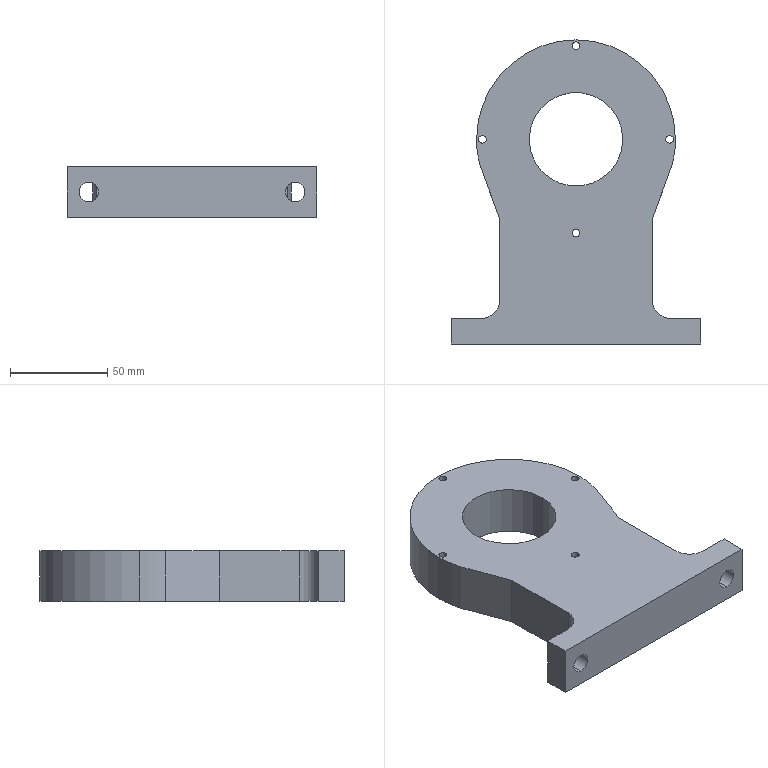Part | NX | features BREP 1 | 1 solid | 32 faces | box 128 x 156 x 26 mm | volume 302066 mm3 | cylinder 19 | plane 13 | commonest cylinder face diameters 4 x8 10 x4 102 x3 20 x2 48 x2
STEP:
#1=CARTESIAN_POINT('',(-50.,32.864,0.));
#2=VERTEX_POINT('',#1);
#3=CARTESIAN_POINT('',(-46.,32.864,0.));
#4=VERTEX_POINT('',#3);
#5=CARTESIAN_POINT('',(-48.,32.864,0.));
#6=DIRECTION('',(0.,0.,1.));
#7=DIRECTION('',(-1.,0.,0.));
#8=AXIS2_PLACEMENT_3D('',#5,#6,#7);
#9=CIRCLE('',#8,2.);
#10=EDGE_CURVE('',#2,#4,#9,.T.);
#11=ORIENTED_EDGE('',*,*,#10,.F.);
#12=CARTESIAN_POINT('',(-50.,32.864,26.));
#13=VERTEX_POINT('',#12);
#14=CARTESIAN_POINT('',(-50.,32.864,-0.001));
#15=DIRECTION('',(0.,0.,1.));
#16=VECTOR('',#15,1000.);
#17=LINE('',#14,#16);
#18=EDGE_CURVE('',#2,#13,#17,.T.);
#19=ORIENTED_EDGE('',*,*,#18,.T.);
#20=CARTESIAN_POINT('',(-46.,32.864,26.));
#21=VERTEX_POINT('',#20);
#22=CARTESIAN_POINT('',(-48.,32.864,26.));
#23=DIRECTION('',(0.,0.,1.));
#24=DIRECTION('',(1.,0.,0.));
#25=AXIS2_PLACEMENT_3D('',#22,#23,#24);
#26=CIRCLE('',#25,2.);
#27=EDGE_CURVE('',#13,#21,#26,.T.);
#28=ORIENTED_EDGE('',*,*,#27,.T.);
#29=CARTESIAN_POINT('',(-46.,32.864,-0.001));
#30=DIRECTION('',(0.,0.,1.));
#31=VECTOR('',#30,1000.);
#32=LINE('',#29,#31);
#33=EDGE_CURVE('',#4,#21,#32,.T.);
#34=ORIENTED_EDGE('',*,*,#33,.F.);
#35=EDGE_LOOP('',(#11,#19,#28,#34));
#36=FACE_BOUND('',#35,.T.);
#37=CARTESIAN_POINT('',(-48.,32.864,-0.001));
#38=DIRECTION('',(0.,0.,1.));
#39=DIRECTION('',(-1.,0.,0.));
#40=AXIS2_PLACEMENT_3D('',#37,#38,#39);
#41=CYLINDRICAL_SURFACE('',#40,2.);
#42=ADVANCED_FACE('',(#36),#41,.F.);
#43=CARTESIAN_POINT('',(-2.,-15.136,0.));
#44=VERTEX_POINT('',#43);
#45=CARTESIAN_POINT('',(2.,-15.136,0.));
#46=VERTEX_POINT('',#45);
#47=CARTESIAN_POINT('',(0.,-15.136,0.));
#48=DIRECTION('',(0.,0.,1.));
#49=DIRECTION('',(-1.,0.,0.));
#50=AXIS2_PLACEMENT_3D('',#47,#48,#49);
#51=CIRCLE('',#50,2.);
#52=EDGE_CURVE('',#44,#46,#51,.T.);
#53=ORIENTED_EDGE('',*,*,#52,.F.);
#54=CARTESIAN_POINT('',(-2.,-15.136,26.));
#55=VERTEX_POINT('',#54);
#56=CARTESIAN_POINT('',(-2.,-15.136,-0.001));
#57=DIRECTION('',(0.,0.,1.));
#58=VECTOR('',#57,1000.);
#59=LINE('',#56,#58);
#60=EDGE_CURVE('',#44,#55,#59,.T.);
#61=ORIENTED_EDGE('',*,*,#60,.T.);
#62=CARTESIAN_POINT('',(2.,-15.136,26.));
#63=VERTEX_POINT('',#62);
#64=CARTESIAN_POINT('',(0.,-15.136,26.));
#65=DIRECTION('',(0.,0.,1.));
#66=DIRECTION('',(1.,0.,0.));
#67=AXIS2_PLACEMENT_3D('',#64,#65,#66);
#68=CIRCLE('',#67,2.);
#69=EDGE_CURVE('',#55,#63,#68,.T.);
#70=ORIENTED_EDGE('',*,*,#69,.T.);
#71=CARTESIAN_POINT('',(2.,-15.136,-0.001));
#72=DIRECTION('',(0.,0.,1.));
#73=VECTOR('',#72,1000.);
#74=LINE('',#71,#73);
#75=EDGE_CURVE('',#46,#63,#74,.T.);
#76=ORIENTED_EDGE('',*,*,#75,.F.);
#77=EDGE_LOOP('',(#53,#61,#70,#76));
#78=FACE_BOUND('',#77,.T.);
#79=CARTESIAN_POINT('',(0.,-15.136,-0.001));
#80=DIRECTION('',(0.,0.,1.));
#81=DIRECTION('',(-1.,0.,0.));
#82=AXIS2_PLACEMENT_3D('',#79,#80,#81);
#83=CYLINDRICAL_SURFACE('',#82,2.);
#84=ADVANCED_FACE('',(#78),#83,.F.);
#85=CARTESIAN_POINT('',(46.,32.864,0.));
#86=VERTEX_POINT('',#85);
#87=CARTESIAN_POINT('',(50.,32.864,0.));
#88=VERTEX_POINT('',#87);
#89=CARTESIAN_POINT('',(48.,32.864,0.));
#90=DIRECTION('',(0.,0.,1.));
#91=DIRECTION('',(-1.,0.,0.));
#92=AXIS2_PLACEMENT_3D('',#89,#90,#91);
#93=CIRCLE('',#92,2.);
#94=EDGE_CURVE('',#86,#88,#93,.T.);
#95=ORIENTED_EDGE('',*,*,#94,.F.);
#96=CARTESIAN_POINT('',(46.,32.864,26.));
#97=VERTEX_POINT('',#96);
#98=CARTESIAN_POINT('',(46.,32.864,-0.001));
#99=DIRECTION('',(0.,0.,1.));
#100=VECTOR('',#99,1000.);
#101=LINE('',#98,#100);
#102=EDGE_CURVE('',#86,#97,#101,.T.);
#103=ORIENTED_EDGE('',*,*,#102,.T.);
#104=CARTESIAN_POINT('',(50.,32.864,26.));
#105=VERTEX_POINT('',#104);
#106=CARTESIAN_POINT('',(48.,32.864,26.));
#107=DIRECTION('',(0.,0.,1.));
#108=DIRECTION('',(1.,0.,0.));
#109=AXIS2_PLACEMENT_3D('',#106,#107,#108);
#110=CIRCLE('',#109,2.);
#111=EDGE_CURVE('',#97,#105,#110,.T.);
#112=ORIENTED_EDGE('',*,*,#111,.T.);
#113=CARTESIAN_POINT('',(50.,32.864,-0.001));
#114=DIRECTION('',(0.,0.,1.));
#115=VECTOR('',#114,1000.);
#116=LINE('',#113,#115);
#117=EDGE_CURVE('',#88,#105,#116,.T.);
#118=ORIENTED_EDGE('',*,*,#117,.F.);
#119=EDGE_LOOP('',(#95,#103,#112,#118));
#120=FACE_BOUND('',#119,.T.);
#121=CARTESIAN_POINT('',(48.,32.864,-0.001));
#122=DIRECTION('',(0.,0.,1.));
#123=DIRECTION('',(-1.,0.,0.));
#124=AXIS2_PLACEMENT_3D('',#121,#122,#123);
#125=CYLINDRICAL_SURFACE('',#124,2.);
#126=ADVANCED_FACE('',(#120),#125,.F.);
#127=CARTESIAN_POINT('',(-2.,80.864,0.));
#128=VERTEX_POINT('',#127);
#129=CARTESIAN_POINT('',(2.,80.864,0.));
#130=VERTEX_POINT('',#129);
#131=CARTESIAN_POINT('',(0.,80.864,0.));
#132=DIRECTION('',(0.,0.,1.));
#133=DIRECTION('',(-1.,0.,0.));
#134=AXIS2_PLACEMENT_3D('',#131,#132,#133);
#135=CIRCLE('',#134,2.);
#136=EDGE_CURVE('',#128,#130,#135,.T.);
#137=ORIENTED_EDGE('',*,*,#136,.F.);
#138=CARTESIAN_POINT('',(-2.,80.864,26.));
#139=VERTEX_POINT('',#138);
#140=CARTESIAN_POINT('',(-2.,80.864,-0.001));
#141=DIRECTION('',(0.,0.,1.));
#142=VECTOR('',#141,1000.);
#143=LINE('',#140,#142);
#144=EDGE_CURVE('',#128,#139,#143,.T.);
#145=ORIENTED_EDGE('',*,*,#144,.T.);
#146=CARTESIAN_POINT('',(2.,80.864,26.));
#147=VERTEX_POINT('',#146);
#148=CARTESIAN_POINT('',(0.,80.864,26.));
#149=DIRECTION('',(0.,0.,1.));
#150=DIRECTION('',(1.,0.,0.));
#151=AXIS2_PLACEMENT_3D('',#148,#149,#150);
#152=CIRCLE('',#151,2.);
#153=EDGE_CURVE('',#139,#147,#152,.T.);
#154=ORIENTED_EDGE('',*,*,#153,.T.);
#155=CARTESIAN_POINT('',(2.,80.864,-0.001));
#156=DIRECTION('',(0.,0.,1.));
#157=VECTOR('',#156,1000.);
#158=LINE('',#155,#157);
#159=EDGE_CURVE('',#130,#147,#158,.T.);
#160=ORIENTED_EDGE('',*,*,#159,.F.);
#161=EDGE_LOOP('',(#137,#145,#154,#160));
#162=FACE_BOUND('',#161,.T.);
#163=CARTESIAN_POINT('',(0.,80.864,-0.001));
#164=DIRECTION('',(0.,0.,1.));
#165=DIRECTION('',(-1.,0.,0.));
#166=AXIS2_PLACEMENT_3D('',#163,#164,#165);
#167=CYLINDRICAL_SURFACE('',#166,2.);
#168=ADVANCED_FACE('',(#162),#167,.F.);
#169=CARTESIAN_POINT('',(53.,-72.136,18.));
#170=VERTEX_POINT('',#169);
#171=CARTESIAN_POINT('',(53.,-72.136,8.));
#172=VERTEX_POINT('',#171);
#173=CARTESIAN_POINT('',(53.,-72.136,13.));
#174=DIRECTION('',(0.,-1.,0.));
#175=DIRECTION('',(0.,0.,1.));
#176=AXIS2_PLACEMENT_3D('',#173,#174,#175);
#177=CIRCLE('',#176,5.);
#178=EDGE_CURVE('',#170,#172,#177,.T.);
#179=ORIENTED_EDGE('',*,*,#178,.T.);
#180=CARTESIAN_POINT('',(53.,-59.136,8.));
#181=VERTEX_POINT('',#180);
#182=CARTESIAN_POINT('',(53.,-72.137,8.));
#183=DIRECTION('',(0.,1.,0.));
#184=VECTOR('',#183,1000.);
#185=LINE('',#182,#184);
#186=EDGE_CURVE('',#172,#181,#185,.T.);
#187=ORIENTED_EDGE('',*,*,#186,.T.);
#188=CARTESIAN_POINT('',(49.,-59.136,10.));
#189=VERTEX_POINT('',#188);
#190=CARTESIAN_POINT('',(53.,-59.136,13.));
#191=DIRECTION('',(0.,1.,0.));
#192=DIRECTION('',(0.,0.,1.));
#193=AXIS2_PLACEMENT_3D('',#190,#191,#192);
#194=CIRCLE('',#193,5.);
#195=EDGE_CURVE('',#181,#189,#194,.T.);
#196=ORIENTED_EDGE('',*,*,#195,.T.);
#197=CARTESIAN_POINT('',(49.,-59.136,16.));
#198=VERTEX_POINT('',#197);
#199=CARTESIAN_POINT('',(53.,-59.136,13.));
#200=DIRECTION('',(0.,1.,0.));
#201=DIRECTION('',(0.,0.,1.));
#202=AXIS2_PLACEMENT_3D('',#199,#200,#201);
#203=CIRCLE('',#202,5.);
#204=EDGE_CURVE('',#189,#198,#203,.T.);
#205=ORIENTED_EDGE('',*,*,#204,.T.);
#206=CARTESIAN_POINT('',(53.,-59.136,18.));
#207=VERTEX_POINT('',#206);
#208=CARTESIAN_POINT('',(53.,-59.136,13.));
#209=DIRECTION('',(0.,1.,0.));
#210=DIRECTION('',(0.,0.,1.));
#211=AXIS2_PLACEMENT_3D('',#208,#209,#210);
#212=CIRCLE('',#211,5.);
#213=EDGE_CURVE('',#198,#207,#212,.T.);
#214=ORIENTED_EDGE('',*,*,#213,.T.);
#215=CARTESIAN_POINT('',(53.,-72.137,18.));
#216=DIRECTION('',(0.,1.,0.));
#217=VECTOR('',#216,1000.);
#218=LINE('',#215,#217);
#219=EDGE_CURVE('',#170,#207,#218,.T.);
#220=ORIENTED_EDGE('',*,*,#219,.F.);
#221=EDGE_LOOP('',(#179,#187,#196,#205,#214,#220));
#222=FACE_BOUND('',#221,.T.);
#223=CARTESIAN_POINT('',(53.,-72.137,13.));
#224=DIRECTION('',(0.,1.,0.));
#225=DIRECTION('',(0.,0.,-1.));
#226=AXIS2_PLACEMENT_3D('',#223,#224,#225);
#227=CYLINDRICAL_SURFACE('',#226,5.);
#228=ADVANCED_FACE('',(#222),#227,.F.);
#229=CARTESIAN_POINT('',(-53.,-72.136,18.));
#230=VERTEX_POINT('',#229);
#231=CARTESIAN_POINT('',(-53.,-72.136,8.));
#232=VERTEX_POINT('',#231);
#233=CARTESIAN_POINT('',(-53.,-72.136,13.));
#234=DIRECTION('',(0.,-1.,0.));
#235=DIRECTION('',(0.,0.,1.));
#236=AXIS2_PLACEMENT_3D('',#233,#234,#235);
#237=CIRCLE('',#236,5.);
#238=EDGE_CURVE('',#230,#232,#237,.T.);
#239=ORIENTED_EDGE('',*,*,#238,.T.);
#240=CARTESIAN_POINT('',(-53.,-59.136,8.));
#241=VERTEX_POINT('',#240);
#242=CARTESIAN_POINT('',(-53.,-72.137,8.));
#243=DIRECTION('',(0.,1.,0.));
#244=VECTOR('',#243,1000.);
#245=LINE('',#242,#244);
#246=EDGE_CURVE('',#232,#241,#245,.T.);
#247=ORIENTED_EDGE('',*,*,#246,.T.);
#248=CARTESIAN_POINT('',(-53.,-59.136,18.));
#249=VERTEX_POINT('',#248);
#250=CARTESIAN_POINT('',(-53.,-59.136,13.));
#251=DIRECTION('',(0.,1.,0.));
#252=DIRECTION('',(0.,0.,1.));
#253=AXIS2_PLACEMENT_3D('',#250,#251,#252);
#254=CIRCLE('',#253,5.);
#255=EDGE_CURVE('',#241,#249,#254,.T.);
#256=ORIENTED_EDGE('',*,*,#255,.T.);
#257=CARTESIAN_POINT('',(-53.,-72.137,18.));
#258=DIRECTION('',(0.,1.,0.));
#259=VECTOR('',#258,1000.);
#260=LINE('',#257,#259);
#261=EDGE_CURVE('',#230,#249,#260,.T.);
#262=ORIENTED_EDGE('',*,*,#261,.F.);
#263=EDGE_LOOP('',(#239,#247,#256,#262));
#264=FACE_BOUND('',#263,.T.);
#265=CARTESIAN_POINT('',(-53.,-72.137,13.));
#266=DIRECTION('',(0.,1.,0.));
#267=DIRECTION('',(0.,0.,-1.));
#268=AXIS2_PLACEMENT_3D('',#265,#266,#267);
#269=CYLINDRICAL_SURFACE('',#268,5.);
#270=ADVANCED_FACE('',(#264),#269,.F.);
#271=CARTESIAN_POINT('',(-24.,32.864,26.));
#272=VERTEX_POINT('',#271);
#273=CARTESIAN_POINT('',(24.,32.864,26.));
#274=VERTEX_POINT('',#273);
#275=CARTESIAN_POINT('',(0.,32.864,26.));
#276=DIRECTION('',(0.,0.,1.));
#277=DIRECTION('',(1.,0.,0.));
#278=AXIS2_PLACEMENT_3D('',#275,#276,#277);
#279=CIRCLE('',#278,24.);
#280=EDGE_CURVE('',#272,#274,#279,.T.);
#281=ORIENTED_EDGE('',*,*,#280,.T.);
#282=CARTESIAN_POINT('',(24.,32.864,0.));
#283=VERTEX_POINT('',#282);
#284=CARTESIAN_POINT('',(24.,32.864,26.));
#285=DIRECTION('',(0.,0.,-1.));
#286=VECTOR('',#285,1000.);
#287=LINE('',#284,#286);
#288=EDGE_CURVE('',#283,#274,#287,.F.);
#289=ORIENTED_EDGE('',*,*,#288,.F.);
#290=CARTESIAN_POINT('',(-24.,32.864,0.));
#291=VERTEX_POINT('',#290);
#292=CARTESIAN_POINT('',(0.,32.864,0.));
#293=DIRECTION('',(0.,0.,1.));
#294=DIRECTION('',(1.,0.,0.));
#295=AXIS2_PLACEMENT_3D('',#292,#293,#294);
#296=CIRCLE('',#295,24.);
#297=EDGE_CURVE('',#291,#283,#296,.T.);
#298=ORIENTED_EDGE('',*,*,#297,.F.);
#299=CARTESIAN_POINT('',(-24.,32.864,26.));
#300=DIRECTION('',(0.,0.,-1.));
#301=VECTOR('',#300,1000.);
#302=LINE('',#299,#301);
#303=EDGE_CURVE('',#291,#272,#302,.F.);
#304=ORIENTED_EDGE('',*,*,#303,.T.);
#305=EDGE_LOOP('',(#281,#289,#298,#304));
#306=FACE_BOUND('',#305,.T.);
#307=CARTESIAN_POINT('',(0.,32.864,26.));
#308=DIRECTION('',(0.,0.,-1.));
#309=DIRECTION('',(1.,0.,0.));
#310=AXIS2_PLACEMENT_3D('',#307,#308,#309);
#311=CYLINDRICAL_SURFACE('',#310,24.);
#312=ADVANCED_FACE('',(#306),#311,.F.);
#313=CARTESIAN_POINT('',(51.,32.864,26.));
#314=VERTEX_POINT('',#313);
#315=CARTESIAN_POINT('',(-51.,32.864,26.));
#316=VERTEX_POINT('',#315);
#317=CARTESIAN_POINT('',(0.,32.864,26.));
#318=DIRECTION('',(0.,0.,1.));
#319=DIRECTION('',(1.,0.,0.));
#320=AXIS2_PLACEMENT_3D('',#317,#318,#319);
#321=CIRCLE('',#320,51.);
#322=EDGE_CURVE('',#314,#316,#321,.T.);
#323=ORIENTED_EDGE('',*,*,#322,.F.);
#324=CARTESIAN_POINT('',(51.,32.864,0.));
#325=VERTEX_POINT('',#324);
#326=CARTESIAN_POINT('',(51.,32.864,26.));
#327=DIRECTION('',(0.,0.,-1.));
#328=VECTOR('',#327,1000.);
#329=LINE('',#326,#328);
#330=EDGE_CURVE('',#314,#325,#329,.T.);
#331=ORIENTED_EDGE('',*,*,#330,.T.);
#332=CARTESIAN_POINT('',(-51.,32.864,0.));
#333=VERTEX_POINT('',#332);
#334=CARTESIAN_POINT('',(0.,32.864,0.));
#335=DIRECTION('',(0.,0.,1.));
#336=DIRECTION('',(1.,0.,0.));
#337=AXIS2_PLACEMENT_3D('',#334,#335,#336);
#338=CIRCLE('',#337,51.);
#339=EDGE_CURVE('',#325,#333,#338,.T.);
#340=ORIENTED_EDGE('',*,*,#339,.T.);
#341=CARTESIAN_POINT('',(-51.,32.864,26.));
#342=DIRECTION('',(0.,0.,-1.));
#343=VECTOR('',#342,1000.);
#344=LINE('',#341,#343);
#345=EDGE_CURVE('',#316,#333,#344,.T.);
#346=ORIENTED_EDGE('',*,*,#345,.F.);
#347=EDGE_LOOP('',(#323,#331,#340,#346));
#348=FACE_BOUND('',#347,.T.);
#349=CARTESIAN_POINT('',(0.,32.864,26.));
#350=DIRECTION('',(0.,0.,-1.));
#351=DIRECTION('',(1.,0.,0.));
#352=AXIS2_PLACEMENT_3D('',#349,#350,#351);
#353=CYLINDRICAL_SURFACE('',#352,51.);
#354=ADVANCED_FACE('',(#348),#353,.T.);
#355=CARTESIAN_POINT('',(-49.179,19.357,26.));
#356=VERTEX_POINT('',#355);
#357=CARTESIAN_POINT('',(0.,32.864,26.));
#358=DIRECTION('',(0.,0.,1.));
#359=DIRECTION('',(1.,0.,0.));
#360=AXIS2_PLACEMENT_3D('',#357,#358,#359);
#361=CIRCLE('',#360,51.);
#362=EDGE_CURVE('',#316,#356,#361,.T.);
#363=ORIENTED_EDGE('',*,*,#362,.F.);
#364=ORIENTED_EDGE('',*,*,#345,.T.);
#365=CARTESIAN_POINT('',(-49.179,19.357,0.));
#366=VERTEX_POINT('',#365);
#367=CARTESIAN_POINT('',(0.,32.864,0.));
#368=DIRECTION('',(0.,0.,1.));
#369=DIRECTION('',(1.,0.,0.));
#370=AXIS2_PLACEMENT_3D('',#367,#368,#369);
#371=CIRCLE('',#370,51.);
#372=EDGE_CURVE('',#333,#366,#371,.T.);
#373=ORIENTED_EDGE('',*,*,#372,.T.);
#374=CARTESIAN_POINT('',(-49.179,19.357,26.));
#375=DIRECTION('',(0.,0.,-1.));
#376=VECTOR('',#375,1000.);
#377=LINE('',#374,#376);
#378=EDGE_CURVE('',#356,#366,#377,.T.);
#379=ORIENTED_EDGE('',*,*,#378,.F.);
#380=EDGE_LOOP('',(#363,#364,#373,#379));
#381=FACE_BOUND('',#380,.T.);
#382=CARTESIAN_POINT('',(0.,32.864,26.));
#383=DIRECTION('',(0.,0.,-1.));
#384=DIRECTION('',(1.,0.,0.));
#385=AXIS2_PLACEMENT_3D('',#382,#383,#384);
#386=CYLINDRICAL_SURFACE('',#385,51.);
#387=ADVANCED_FACE('',(#381),#386,.T.);
#388=CARTESIAN_POINT('',(39.,-49.136,26.));
#389=VERTEX_POINT('',#388);
#390=CARTESIAN_POINT('',(39.,-8.136,26.));
#391=VERTEX_POINT('',#390);
#392=CARTESIAN_POINT('',(39.,-8.136,26.));
#393=DIRECTION('',(0.,1.,0.));
#394=VECTOR('',#393,1000.);
#395=LINE('',#392,#394);
#396=EDGE_CURVE('',#389,#391,#395,.T.);
#397=ORIENTED_EDGE('',*,*,#396,.T.);
#398=CARTESIAN_POINT('',(49.179,19.357,26.));
#399=VERTEX_POINT('',#398);
#400=CARTESIAN_POINT('',(39.,-8.136,26.));
#401=DIRECTION('',(0.3472,0.9378,0.));
#402=VECTOR('',#401,1000.);
#403=LINE('',#400,#402);
#404=EDGE_CURVE('',#391,#399,#403,.T.);
#405=ORIENTED_EDGE('',*,*,#404,.T.);
#406=CARTESIAN_POINT('',(0.,32.864,26.));
#407=DIRECTION('',(0.,0.,1.));
#408=DIRECTION('',(1.,0.,0.));
#409=AXIS2_PLACEMENT_3D('',#406,#407,#408);
#410=CIRCLE('',#409,51.);
#411=EDGE_CURVE('',#399,#314,#410,.T.);
#412=ORIENTED_EDGE('',*,*,#411,.T.);
#413=ORIENTED_EDGE('',*,*,#322,.T.);
#414=ORIENTED_EDGE('',*,*,#362,.T.);
#415=CARTESIAN_POINT('',(-39.,-8.136,26.));
#416=VERTEX_POINT('',#415);
#417=CARTESIAN_POINT('',(-39.,-8.136,26.));
#418=DIRECTION('',(0.3472,-0.9378,0.));
#419=VECTOR('',#418,1000.);
#420=LINE('',#417,#419);
#421=EDGE_CURVE('',#356,#416,#420,.T.);
#422=ORIENTED_EDGE('',*,*,#421,.T.);
#423=CARTESIAN_POINT('',(-39.,-49.136,26.));
#424=VERTEX_POINT('',#423);
#425=CARTESIAN_POINT('',(-39.,-8.136,26.));
#426=DIRECTION('',(0.,-1.,0.));
#427=VECTOR('',#426,1000.);
#428=LINE('',#425,#427);
#429=EDGE_CURVE('',#416,#424,#428,.T.);
#430=ORIENTED_EDGE('',*,*,#429,.T.);
#431=CARTESIAN_POINT('',(-49.,-59.136,26.));
#432=VERTEX_POINT('',#431);
#433=CARTESIAN_POINT('',(-49.,-49.136,26.));
#434=DIRECTION('',(0.,0.,-1.));
#435=DIRECTION('',(1.,0.,0.));
#436=AXIS2_PLACEMENT_3D('',#433,#434,#435);
#437=CIRCLE('',#436,10.);
#438=EDGE_CURVE('',#424,#432,#437,.T.);
#439=ORIENTED_EDGE('',*,*,#438,.T.);
#440=CARTESIAN_POINT('',(-64.,-59.136,26.));
#441=VERTEX_POINT('',#440);
#442=CARTESIAN_POINT('',(-64.,-59.136,26.));
#443=DIRECTION('',(-1.,0.,0.));
#444=VECTOR('',#443,1000.);
#445=LINE('',#442,#444);
#446=EDGE_CURVE('',#432,#441,#445,.T.);
#447=ORIENTED_EDGE('',*,*,#446,.T.);
#448=CARTESIAN_POINT('',(-64.,-72.136,26.));
#449=VERTEX_POINT('',#448);
#450=CARTESIAN_POINT('',(-64.,-72.136,26.));
#451=DIRECTION('',(0.,-1.,0.));
#452=VECTOR('',#451,1000.);
#453=LINE('',#450,#452);
#454=EDGE_CURVE('',#441,#449,#453,.T.);
#455=ORIENTED_EDGE('',*,*,#454,.T.);
#456=CARTESIAN_POINT('',(64.,-72.136,26.));
#457=VERTEX_POINT('',#456);
#458=CARTESIAN_POINT('',(-64.,-72.136,26.));
#459=DIRECTION('',(1.,0.,0.));
#460=VECTOR('',#459,1000.);
#461=LINE('',#458,#460);
#462=EDGE_CURVE('',#449,#457,#461,.T.);
#463=ORIENTED_EDGE('',*,*,#462,.T.);
#464=CARTESIAN_POINT('',(64.,-59.136,26.));
#465=VERTEX_POINT('',#464);
#466=CARTESIAN_POINT('',(64.,-72.136,26.));
#467=DIRECTION('',(0.,1.,0.));
#468=VECTOR('',#467,1000.);
#469=LINE('',#466,#468);
#470=EDGE_CURVE('',#457,#465,#469,.T.);
#471=ORIENTED_EDGE('',*,*,#470,.T.);
#472=CARTESIAN_POINT('',(49.,-59.136,26.));
#473=VERTEX_POINT('',#472);
#474=CARTESIAN_POINT('',(49.,-59.136,26.));
#475=DIRECTION('',(-1.,0.,0.));
#476=VECTOR('',#475,1000.);
#477=LINE('',#474,#476);
#478=EDGE_CURVE('',#465,#473,#477,.T.);
#479=ORIENTED_EDGE('',*,*,#478,.T.);
#480=CARTESIAN_POINT('',(49.,-49.136,26.));
#481=DIRECTION('',(0.,0.,-1.));
#482=DIRECTION('',(-1.,0.,0.));
#483=AXIS2_PLACEMENT_3D('',#480,#481,#482);
#484=CIRCLE('',#483,10.);
#485=EDGE_CURVE('',#473,#389,#484,.T.);
#486=ORIENTED_EDGE('',*,*,#485,.T.);
#487=EDGE_LOOP('',(#397,#405,#412,#413,#414,#422,#430,#439,#447,#455,#463,#471,#479,#486));
#488=FACE_BOUND('',#487,.T.);
#489=CARTESIAN_POINT('',(-48.,32.864,26.));
#490=DIRECTION('',(0.,0.,1.));
#491=DIRECTION('',(1.,0.,0.));
#492=AXIS2_PLACEMENT_3D('',#489,#490,#491);
#493=CIRCLE('',#492,2.);
#494=EDGE_CURVE('',#21,#13,#493,.T.);
#495=ORIENTED_EDGE('',*,*,#494,.F.);
#496=ORIENTED_EDGE('',*,*,#27,.F.);
#497=EDGE_LOOP('',(#495,#496));
#498=FACE_BOUND('',#497,.T.);
#499=CARTESIAN_POINT('',(0.,-15.136,26.));
#500=DIRECTION('',(0.,0.,1.));
#501=DIRECTION('',(1.,0.,0.));
#502=AXIS2_PLACEMENT_3D('',#499,#500,#501);
#503=CIRCLE('',#502,2.);
#504=EDGE_CURVE('',#63,#55,#503,.T.);
#505=ORIENTED_EDGE('',*,*,#504,.F.);
#506=ORIENTED_EDGE('',*,*,#69,.F.);
#507=EDGE_LOOP('',(#505,#506));
#508=FACE_BOUND('',#507,.T.);
#509=CARTESIAN_POINT('',(48.,32.864,26.));
#510=DIRECTION('',(0.,0.,1.));
#511=DIRECTION('',(1.,0.,0.));
#512=AXIS2_PLACEMENT_3D('',#509,#510,#511);
#513=CIRCLE('',#512,2.);
#514=EDGE_CURVE('',#105,#97,#513,.T.);
#515=ORIENTED_EDGE('',*,*,#514,.F.);
#516=ORIENTED_EDGE('',*,*,#111,.F.);
#517=EDGE_LOOP('',(#515,#516));
#518=FACE_BOUND('',#517,.T.);
#519=CARTESIAN_POINT('',(0.,80.864,26.));
#520=DIRECTION('',(0.,0.,1.));
#521=DIRECTION('',(1.,0.,0.));
#522=AXIS2_PLACEMENT_3D('',#519,#520,#521);
#523=CIRCLE('',#522,2.);
#524=EDGE_CURVE('',#147,#139,#523,.T.);
#525=ORIENTED_EDGE('',*,*,#524,.F.);
#526=ORIENTED_EDGE('',*,*,#153,.F.);
#527=EDGE_LOOP('',(#525,#526));
#528=FACE_BOUND('',#527,.T.);
#529=ORIENTED_EDGE('',*,*,#280,.F.);
#530=CARTESIAN_POINT('',(0.,32.864,26.));
#531=DIRECTION('',(0.,0.,1.));
#532=DIRECTION('',(1.,0.,0.));
#533=AXIS2_PLACEMENT_3D('',#530,#531,#532);
#534=CIRCLE('',#533,24.);
#535=EDGE_CURVE('',#274,#272,#534,.T.);
#536=ORIENTED_EDGE('',*,*,#535,.F.);
#537=EDGE_LOOP('',(#529,#536));
#538=FACE_BOUND('',#537,.T.);
#539=CARTESIAN_POINT('',(49.,-49.136,26.));
#540=DIRECTION('',(0.,0.,-1.));
#541=DIRECTION('',(0.,1.,0.));
#542=AXIS2_PLACEMENT_3D('',#539,#540,#541);
#543=PLANE('',#542);
#544=ADVANCED_FACE('',(#488,#498,#508,#518,#528,#538),#543,.F.);
#545=CARTESIAN_POINT('',(39.,-49.136,0.));
#546=VERTEX_POINT('',#545);
#547=CARTESIAN_POINT('',(39.,-8.136,0.));
#548=VERTEX_POINT('',#547);
#549=CARTESIAN_POINT('',(39.,-8.136,0.));
#550=DIRECTION('',(0.,1.,0.));
#551=VECTOR('',#550,1000.);
#552=LINE('',#549,#551);
#553=EDGE_CURVE('',#546,#548,#552,.T.);
#554=ORIENTED_EDGE('',*,*,#553,.F.);
#555=CARTESIAN_POINT('',(49.,-59.136,0.));
#556=VERTEX_POINT('',#555);
#557=CARTESIAN_POINT('',(49.,-49.136,0.));
#558=DIRECTION('',(0.,0.,-1.));
#559=DIRECTION('',(-1.,0.,0.));
#560=AXIS2_PLACEMENT_3D('',#557,#558,#559);
#561=CIRCLE('',#560,10.);
#562=EDGE_CURVE('',#556,#546,#561,.T.);
#563=ORIENTED_EDGE('',*,*,#562,.F.);
#564=CARTESIAN_POINT('',(64.,-59.136,0.));
#565=VERTEX_POINT('',#564);
#566=CARTESIAN_POINT('',(49.,-59.136,0.));
#567=DIRECTION('',(-1.,0.,0.));
#568=VECTOR('',#567,1000.);
#569=LINE('',#566,#568);
#570=EDGE_CURVE('',#565,#556,#569,.T.);
#571=ORIENTED_EDGE('',*,*,#570,.F.);
#572=CARTESIAN_POINT('',(64.,-72.136,0.));
#573=VERTEX_POINT('',#572);
#574=CARTESIAN_POINT('',(64.,-72.136,0.));
#575=DIRECTION('',(0.,1.,0.));
#576=VECTOR('',#575,1000.);
#577=LINE('',#574,#576);
#578=EDGE_CURVE('',#573,#565,#577,.T.);
#579=ORIENTED_EDGE('',*,*,#578,.F.);
#580=CARTESIAN_POINT('',(-64.,-72.136,0.));
#581=VERTEX_POINT('',#580);
#582=CARTESIAN_POINT('',(-64.,-72.136,0.));
#583=DIRECTION('',(1.,0.,0.));
#584=VECTOR('',#583,1000.);
#585=LINE('',#582,#584);
#586=EDGE_CURVE('',#581,#573,#585,.T.);
#587=ORIENTED_EDGE('',*,*,#586,.F.);
#588=CARTESIAN_POINT('',(-64.,-59.136,0.));
#589=VERTEX_POINT('',#588);
#590=CARTESIAN_POINT('',(-64.,-72.136,0.));
#591=DIRECTION('',(0.,-1.,0.));
#592=VECTOR('',#591,1000.);
#593=LINE('',#590,#592);
#594=EDGE_CURVE('',#589,#581,#593,.T.);
#595=ORIENTED_EDGE('',*,*,#594,.F.);
#596=CARTESIAN_POINT('',(-49.,-59.136,0.));
#597=VERTEX_POINT('',#596);
#598=CARTESIAN_POINT('',(-64.,-59.136,0.));
#599=DIRECTION('',(-1.,0.,0.));
#600=VECTOR('',#599,1000.);
#601=LINE('',#598,#600);
#602=EDGE_CURVE('',#597,#589,#601,.T.);
#603=ORIENTED_EDGE('',*,*,#602,.F.);
#604=CARTESIAN_POINT('',(-39.,-49.136,0.));
#605=VERTEX_POINT('',#604);
#606=CARTESIAN_POINT('',(-49.,-49.136,0.));
#607=DIRECTION('',(0.,0.,-1.));
#608=DIRECTION('',(1.,0.,0.));
#609=AXIS2_PLACEMENT_3D('',#606,#607,#608);
#610=CIRCLE('',#609,10.);
#611=EDGE_CURVE('',#605,#597,#610,.T.);
#612=ORIENTED_EDGE('',*,*,#611,.F.);
#613=CARTESIAN_POINT('',(-39.,-8.136,0.));
#614=VERTEX_POINT('',#613);
#615=CARTESIAN_POINT('',(-39.,-8.136,0.));
#616=DIRECTION('',(0.,-1.,0.));
#617=VECTOR('',#616,1000.);
#618=LINE('',#615,#617);
#619=EDGE_CURVE('',#614,#605,#618,.T.);
#620=ORIENTED_EDGE('',*,*,#619,.F.);
#621=CARTESIAN_POINT('',(-39.,-8.136,0.));
#622=DIRECTION('',(0.3472,-0.9378,0.));
#623=VECTOR('',#622,1000.);
#624=LINE('',#621,#623);
#625=EDGE_CURVE('',#366,#614,#624,.T.);
#626=ORIENTED_EDGE('',*,*,#625,.F.);
#627=ORIENTED_EDGE('',*,*,#372,.F.);
#628=ORIENTED_EDGE('',*,*,#339,.F.);
#629=CARTESIAN_POINT('',(49.179,19.357,0.));
#630=VERTEX_POINT('',#629);
#631=CARTESIAN_POINT('',(0.,32.864,0.));
#632=DIRECTION('',(0.,0.,1.));
#633=DIRECTION('',(1.,0.,0.));
#634=AXIS2_PLACEMENT_3D('',#631,#632,#633);
#635=CIRCLE('',#634,51.);
#636=EDGE_CURVE('',#630,#325,#635,.T.);
#637=ORIENTED_EDGE('',*,*,#636,.F.);
#638=CARTESIAN_POINT('',(39.,-8.136,0.));
#639=DIRECTION('',(0.3472,0.9378,0.));
#640=VECTOR('',#639,1000.);
#641=LINE('',#638,#640);
#642=EDGE_CURVE('',#548,#630,#641,.T.);
#643=ORIENTED_EDGE('',*,*,#642,.F.);
#644=EDGE_LOOP('',(#554,#563,#571,#579,#587,#595,#603,#612,#620,#626,#627,#628,#637,#643));
#645=FACE_BOUND('',#644,.T.);
#646=CARTESIAN_POINT('',(-48.,32.864,0.));
#647=DIRECTION('',(0.,0.,1.));
#648=DIRECTION('',(-1.,0.,0.));
#649=AXIS2_PLACEMENT_3D('',#646,#647,#648);
#650=CIRCLE('',#649,2.);
#651=EDGE_CURVE('',#4,#2,#650,.T.);
#652=ORIENTED_EDGE('',*,*,#651,.T.);
#653=ORIENTED_EDGE('',*,*,#10,.T.);
#654=EDGE_LOOP('',(#652,#653));
#655=FACE_BOUND('',#654,.T.);
#656=CARTESIAN_POINT('',(0.,-15.136,0.));
#657=DIRECTION('',(0.,0.,1.));
#658=DIRECTION('',(-1.,0.,0.));
#659=AXIS2_PLACEMENT_3D('',#656,#657,#658);
#660=CIRCLE('',#659,2.);
#661=EDGE_CURVE('',#46,#44,#660,.T.);
#662=ORIENTED_EDGE('',*,*,#661,.T.);
#663=ORIENTED_EDGE('',*,*,#52,.T.);
#664=EDGE_LOOP('',(#662,#663));
#665=FACE_BOUND('',#664,.T.);
#666=CARTESIAN_POINT('',(48.,32.864,0.));
#667=DIRECTION('',(0.,0.,1.));
#668=DIRECTION('',(-1.,0.,0.));
#669=AXIS2_PLACEMENT_3D('',#666,#667,#668);
#670=CIRCLE('',#669,2.);
#671=EDGE_CURVE('',#88,#86,#670,.T.);
#672=ORIENTED_EDGE('',*,*,#671,.T.);
#673=ORIENTED_EDGE('',*,*,#94,.T.);
#674=EDGE_LOOP('',(#672,#673));
#675=FACE_BOUND('',#674,.T.);
#676=CARTESIAN_POINT('',(0.,80.864,0.));
#677=DIRECTION('',(0.,0.,1.));
#678=DIRECTION('',(-1.,0.,0.));
#679=AXIS2_PLACEMENT_3D('',#676,#677,#678);
#680=CIRCLE('',#679,2.);
#681=EDGE_CURVE('',#130,#128,#680,.T.);
#682=ORIENTED_EDGE('',*,*,#681,.T.);
#683=ORIENTED_EDGE('',*,*,#136,.T.);
#684=EDGE_LOOP('',(#682,#683));
#685=FACE_BOUND('',#684,.T.);
#686=ORIENTED_EDGE('',*,*,#297,.T.);
#687=CARTESIAN_POINT('',(0.,32.864,0.));
#688=DIRECTION('',(0.,0.,1.));
#689=DIRECTION('',(1.,0.,0.));
#690=AXIS2_PLACEMENT_3D('',#687,#688,#689);
#691=CIRCLE('',#690,24.);
#692=EDGE_CURVE('',#283,#291,#691,.T.);
#693=ORIENTED_EDGE('',*,*,#692,.T.);
#694=EDGE_LOOP('',(#686,#693));
#695=FACE_BOUND('',#694,.T.);
#696=CARTESIAN_POINT('',(49.,-49.136,0.));
#697=DIRECTION('',(0.,0.,-1.));
#698=DIRECTION('',(0.,1.,0.));
#699=AXIS2_PLACEMENT_3D('',#696,#697,#698);
#700=PLANE('',#699);
#701=ADVANCED_FACE('',(#645,#655,#665,#675,#685,#695),#700,.T.);
#702=ORIENTED_EDGE('',*,*,#553,.T.);
#703=CARTESIAN_POINT('',(39.,-8.136,26.));
#704=DIRECTION('',(0.,0.,-1.));
#705=VECTOR('',#704,1000.);
#706=LINE('',#703,#705);
#707=EDGE_CURVE('',#391,#548,#706,.T.);
#708=ORIENTED_EDGE('',*,*,#707,.F.);
#709=ORIENTED_EDGE('',*,*,#396,.F.);
#710=CARTESIAN_POINT('',(39.,-49.136,26.));
#711=DIRECTION('',(0.,0.,-1.));
#712=VECTOR('',#711,1000.);
#713=LINE('',#710,#712);
#714=EDGE_CURVE('',#389,#546,#713,.T.);
#715=ORIENTED_EDGE('',*,*,#714,.T.);
#716=EDGE_LOOP('',(#702,#708,#709,#715));
#717=FACE_BOUND('',#716,.T.);
#718=CARTESIAN_POINT('',(39.,-8.136,26.));
#719=DIRECTION('',(-1.,0.,0.));
#720=DIRECTION('',(0.,-1.,0.));
#721=AXIS2_PLACEMENT_3D('',#718,#719,#720);
#722=PLANE('',#721);
#723=ADVANCED_FACE('',(#717),#722,.F.);
#724=ORIENTED_EDGE('',*,*,#642,.T.);
#725=CARTESIAN_POINT('',(49.179,19.357,26.));
#726=DIRECTION('',(0.,0.,-1.));
#727=VECTOR('',#726,1000.);
#728=LINE('',#725,#727);
#729=EDGE_CURVE('',#399,#630,#728,.T.);
#730=ORIENTED_EDGE('',*,*,#729,.F.);
#731=ORIENTED_EDGE('',*,*,#404,.F.);
#732=ORIENTED_EDGE('',*,*,#707,.T.);
#733=EDGE_LOOP('',(#724,#730,#731,#732));
#734=FACE_BOUND('',#733,.T.);
#735=CARTESIAN_POINT('',(39.,-8.136,26.));
#736=DIRECTION('',(-0.9378,0.3472,0.));
#737=DIRECTION('',(0.,0.,-1.));
#738=AXIS2_PLACEMENT_3D('',#735,#736,#737);
#739=PLANE('',#738);
#740=ADVANCED_FACE('',(#734),#739,.F.);
#741=ORIENTED_EDGE('',*,*,#330,.F.);
#742=ORIENTED_EDGE('',*,*,#411,.F.);
#743=ORIENTED_EDGE('',*,*,#729,.T.);
#744=ORIENTED_EDGE('',*,*,#636,.T.);
#745=EDGE_LOOP('',(#741,#742,#743,#744));
#746=FACE_BOUND('',#745,.T.);
#747=CARTESIAN_POINT('',(0.,32.864,26.));
#748=DIRECTION('',(0.,0.,-1.));
#749=DIRECTION('',(1.,0.,0.));
#750=AXIS2_PLACEMENT_3D('',#747,#748,#749);
#751=CYLINDRICAL_SURFACE('',#750,51.);
#752=ADVANCED_FACE('',(#746),#751,.T.);
#753=ORIENTED_EDGE('',*,*,#625,.T.);
#754=CARTESIAN_POINT('',(-39.,-8.136,26.));
#755=DIRECTION('',(0.,0.,-1.));
#756=VECTOR('',#755,1000.);
#757=LINE('',#754,#756);
#758=EDGE_CURVE('',#416,#614,#757,.T.);
#759=ORIENTED_EDGE('',*,*,#758,.F.);
#760=ORIENTED_EDGE('',*,*,#421,.F.);
#761=ORIENTED_EDGE('',*,*,#378,.T.);
#762=EDGE_LOOP('',(#753,#759,#760,#761));
#763=FACE_BOUND('',#762,.T.);
#764=CARTESIAN_POINT('',(-39.,-8.136,26.));
#765=DIRECTION('',(0.9378,0.3472,0.));
#766=DIRECTION('',(0.,0.,1.));
#767=AXIS2_PLACEMENT_3D('',#764,#765,#766);
#768=PLANE('',#767);
#769=ADVANCED_FACE('',(#763),#768,.F.);
#770=ORIENTED_EDGE('',*,*,#619,.T.);
#771=CARTESIAN_POINT('',(-39.,-49.136,26.));
#772=DIRECTION('',(0.,0.,-1.));
#773=VECTOR('',#772,1000.);
#774=LINE('',#771,#773);
#775=EDGE_CURVE('',#424,#605,#774,.T.);
#776=ORIENTED_EDGE('',*,*,#775,.F.);
#777=ORIENTED_EDGE('',*,*,#429,.F.);
#778=ORIENTED_EDGE('',*,*,#758,.T.);
#779=EDGE_LOOP('',(#770,#776,#777,#778));
#780=FACE_BOUND('',#779,.T.);
#781=CARTESIAN_POINT('',(-39.,-8.136,26.));
#782=DIRECTION('',(1.,0.,0.));
#783=DIRECTION('',(0.,-1.,0.));
#784=AXIS2_PLACEMENT_3D('',#781,#782,#783);
#785=PLANE('',#784);
#786=ADVANCED_FACE('',(#780),#785,.F.);
#787=ORIENTED_EDGE('',*,*,#611,.T.);
#788=CARTESIAN_POINT('',(-49.,-59.136,10.));
#789=VERTEX_POINT('',#788);
#790=CARTESIAN_POINT('',(-49.,-59.136,26.));
#791=DIRECTION('',(0.,0.,-1.));
#792=VECTOR('',#791,1000.);
#793=LINE('',#790,#792);
#794=EDGE_CURVE('',#789,#597,#793,.T.);
#795=ORIENTED_EDGE('',*,*,#794,.F.);
#796=CARTESIAN_POINT('',(-49.,-59.136,16.));
#797=VERTEX_POINT('',#796);
#798=CARTESIAN_POINT('',(-49.,-59.136,26.));
#799=DIRECTION('',(0.,0.,-1.));
#800=VECTOR('',#799,1000.);
#801=LINE('',#798,#800);
#802=EDGE_CURVE('',#797,#789,#801,.T.);
#803=ORIENTED_EDGE('',*,*,#802,.F.);
#804=CARTESIAN_POINT('',(-49.,-59.136,26.));
#805=DIRECTION('',(0.,0.,-1.));
#806=VECTOR('',#805,1000.);
#807=LINE('',#804,#806);
#808=EDGE_CURVE('',#432,#797,#807,.T.);
#809=ORIENTED_EDGE('',*,*,#808,.F.);
#810=ORIENTED_EDGE('',*,*,#438,.F.);
#811=ORIENTED_EDGE('',*,*,#775,.T.);
#812=EDGE_LOOP('',(#787,#795,#803,#809,#810,#811));
#813=FACE_BOUND('',#812,.T.);
#814=CARTESIAN_POINT('',(-49.,-49.136,26.));
#815=DIRECTION('',(0.,0.,-1.));
#816=DIRECTION('',(1.,0.,0.));
#817=AXIS2_PLACEMENT_3D('',#814,#815,#816);
#818=CYLINDRICAL_SURFACE('',#817,10.);
#819=ADVANCED_FACE('',(#813),#818,.F.);
#820=ORIENTED_EDGE('',*,*,#808,.T.);
#821=CARTESIAN_POINT('',(-53.,-59.136,13.));
#822=DIRECTION('',(0.,1.,0.));
#823=DIRECTION('',(0.,0.,1.));
#824=AXIS2_PLACEMENT_3D('',#821,#822,#823);
#825=CIRCLE('',#824,5.);
#826=EDGE_CURVE('',#249,#797,#825,.T.);
#827=ORIENTED_EDGE('',*,*,#826,.F.);
#828=ORIENTED_EDGE('',*,*,#255,.F.);
#829=CARTESIAN_POINT('',(-53.,-59.136,13.));
#830=DIRECTION('',(0.,1.,0.));
#831=DIRECTION('',(0.,0.,1.));
#832=AXIS2_PLACEMENT_3D('',#829,#830,#831);
#833=CIRCLE('',#832,5.);
#834=EDGE_CURVE('',#789,#241,#833,.T.);
#835=ORIENTED_EDGE('',*,*,#834,.F.);
#836=ORIENTED_EDGE('',*,*,#794,.T.);
#837=ORIENTED_EDGE('',*,*,#602,.T.);
#838=CARTESIAN_POINT('',(-64.,-59.136,26.));
#839=DIRECTION('',(0.,0.,-1.));
#840=VECTOR('',#839,1000.);
#841=LINE('',#838,#840);
#842=EDGE_CURVE('',#441,#589,#841,.T.);
#843=ORIENTED_EDGE('',*,*,#842,.F.);
#844=ORIENTED_EDGE('',*,*,#446,.F.);
#845=EDGE_LOOP('',(#820,#827,#828,#835,#836,#837,#843,#844));
#846=FACE_BOUND('',#845,.T.);
#847=CARTESIAN_POINT('',(-64.,-59.136,26.));
#848=DIRECTION('',(0.,-1.,0.));
#849=DIRECTION('',(0.,0.,1.));
#850=AXIS2_PLACEMENT_3D('',#847,#848,#849);
#851=PLANE('',#850);
#852=ADVANCED_FACE('',(#846),#851,.F.);
#853=ORIENTED_EDGE('',*,*,#594,.T.);
#854=CARTESIAN_POINT('',(-64.,-72.136,26.));
#855=DIRECTION('',(0.,0.,-1.));
#856=VECTOR('',#855,1000.);
#857=LINE('',#854,#856);
#858=EDGE_CURVE('',#449,#581,#857,.T.);
#859=ORIENTED_EDGE('',*,*,#858,.F.);
#860=ORIENTED_EDGE('',*,*,#454,.F.);
#861=ORIENTED_EDGE('',*,*,#842,.T.);
#862=EDGE_LOOP('',(#853,#859,#860,#861));
#863=FACE_BOUND('',#862,.T.);
#864=CARTESIAN_POINT('',(-64.,-72.136,26.));
#865=DIRECTION('',(1.,0.,0.));
#866=DIRECTION('',(0.,-1.,0.));
#867=AXIS2_PLACEMENT_3D('',#864,#865,#866);
#868=PLANE('',#867);
#869=ADVANCED_FACE('',(#863),#868,.F.);
#870=ORIENTED_EDGE('',*,*,#586,.T.);
#871=CARTESIAN_POINT('',(64.,-72.136,26.));
#872=DIRECTION('',(0.,0.,-1.));
#873=VECTOR('',#872,1000.);
#874=LINE('',#871,#873);
#875=EDGE_CURVE('',#457,#573,#874,.T.);
#876=ORIENTED_EDGE('',*,*,#875,.F.);
#877=ORIENTED_EDGE('',*,*,#462,.F.);
#878=ORIENTED_EDGE('',*,*,#858,.T.);
#879=EDGE_LOOP('',(#870,#876,#877,#878));
#880=FACE_BOUND('',#879,.T.);
#881=ORIENTED_EDGE('',*,*,#178,.F.);
#882=CARTESIAN_POINT('',(53.,-72.136,13.));
#883=DIRECTION('',(0.,-1.,0.));
#884=DIRECTION('',(0.,0.,1.));
#885=AXIS2_PLACEMENT_3D('',#882,#883,#884);
#886=CIRCLE('',#885,5.);
#887=EDGE_CURVE('',#172,#170,#886,.T.);
#888=ORIENTED_EDGE('',*,*,#887,.F.);
#889=EDGE_LOOP('',(#881,#888));
#890=FACE_BOUND('',#889,.T.);
#891=ORIENTED_EDGE('',*,*,#238,.F.);
#892=CARTESIAN_POINT('',(-53.,-72.136,13.));
#893=DIRECTION('',(0.,-1.,0.));
#894=DIRECTION('',(0.,0.,1.));
#895=AXIS2_PLACEMENT_3D('',#892,#893,#894);
#896=CIRCLE('',#895,5.);
#897=EDGE_CURVE('',#232,#230,#896,.T.);
#898=ORIENTED_EDGE('',*,*,#897,.F.);
#899=EDGE_LOOP('',(#891,#898));
#900=FACE_BOUND('',#899,.T.);
#901=CARTESIAN_POINT('',(-64.,-72.136,26.));
#902=DIRECTION('',(0.,1.,0.));
#903=DIRECTION('',(-1.,0.,0.));
#904=AXIS2_PLACEMENT_3D('',#901,#902,#903);
#905=PLANE('',#904);
#906=ADVANCED_FACE('',(#880,#890,#900),#905,.F.);
#907=ORIENTED_EDGE('',*,*,#578,.T.);
#908=CARTESIAN_POINT('',(64.,-59.136,26.));
#909=DIRECTION('',(0.,0.,-1.));
#910=VECTOR('',#909,1000.);
#911=LINE('',#908,#910);
#912=EDGE_CURVE('',#465,#565,#911,.T.);
#913=ORIENTED_EDGE('',*,*,#912,.F.);
#914=ORIENTED_EDGE('',*,*,#470,.F.);
#915=ORIENTED_EDGE('',*,*,#875,.T.);
#916=EDGE_LOOP('',(#907,#913,#914,#915));
#917=FACE_BOUND('',#916,.T.);
#918=CARTESIAN_POINT('',(64.,-72.136,26.));
#919=DIRECTION('',(-1.,0.,0.));
#920=DIRECTION('',(0.,-1.,0.));
#921=AXIS2_PLACEMENT_3D('',#918,#919,#920);
#922=PLANE('',#921);
#923=ADVANCED_FACE('',(#917),#922,.F.);
#924=CARTESIAN_POINT('',(49.,-59.136,26.));
#925=DIRECTION('',(0.,0.,-1.));
#926=VECTOR('',#925,1000.);
#927=LINE('',#924,#926);
#928=EDGE_CURVE('',#189,#556,#927,.T.);
#929=ORIENTED_EDGE('',*,*,#928,.F.);
#930=ORIENTED_EDGE('',*,*,#195,.F.);
#931=CARTESIAN_POINT('',(53.,-59.136,13.));
#932=DIRECTION('',(0.,1.,0.));
#933=DIRECTION('',(0.,0.,1.));
#934=AXIS2_PLACEMENT_3D('',#931,#932,#933);
#935=CIRCLE('',#934,5.);
#936=EDGE_CURVE('',#207,#181,#935,.T.);
#937=ORIENTED_EDGE('',*,*,#936,.F.);
#938=ORIENTED_EDGE('',*,*,#213,.F.);
#939=CARTESIAN_POINT('',(49.,-59.136,26.));
#940=DIRECTION('',(0.,0.,-1.));
#941=VECTOR('',#940,1000.);
#942=LINE('',#939,#941);
#943=EDGE_CURVE('',#473,#198,#942,.T.);
#944=ORIENTED_EDGE('',*,*,#943,.F.);
#945=ORIENTED_EDGE('',*,*,#478,.F.);
#946=ORIENTED_EDGE('',*,*,#912,.T.);
#947=ORIENTED_EDGE('',*,*,#570,.T.);
#948=EDGE_LOOP('',(#929,#930,#937,#938,#944,#945,#946,#947));
#949=FACE_BOUND('',#948,.T.);
#950=CARTESIAN_POINT('',(49.,-59.136,26.));
#951=DIRECTION('',(0.,-1.,0.));
#952=DIRECTION('',(0.,0.,1.));
#953=AXIS2_PLACEMENT_3D('',#950,#951,#952);
#954=PLANE('',#953);
#955=ADVANCED_FACE('',(#949),#954,.F.);
#956=ORIENTED_EDGE('',*,*,#562,.T.);
#957=ORIENTED_EDGE('',*,*,#714,.F.);
#958=ORIENTED_EDGE('',*,*,#485,.F.);
#959=ORIENTED_EDGE('',*,*,#943,.T.);
#960=CARTESIAN_POINT('',(49.,-59.136,26.));
#961=DIRECTION('',(0.,0.,-1.));
#962=VECTOR('',#961,1000.);
#963=LINE('',#960,#962);
#964=EDGE_CURVE('',#198,#189,#963,.T.);
#965=ORIENTED_EDGE('',*,*,#964,.T.);
#966=ORIENTED_EDGE('',*,*,#928,.T.);
#967=EDGE_LOOP('',(#956,#957,#958,#959,#965,#966));
#968=FACE_BOUND('',#967,.T.);
#969=CARTESIAN_POINT('',(49.,-49.136,26.));
#970=DIRECTION('',(0.,0.,-1.));
#971=DIRECTION('',(1.,0.,0.));
#972=AXIS2_PLACEMENT_3D('',#969,#970,#971);
#973=CYLINDRICAL_SURFACE('',#972,10.);
#974=ADVANCED_FACE('',(#968),#973,.F.);
#975=ORIENTED_EDGE('',*,*,#288,.T.);
#976=ORIENTED_EDGE('',*,*,#535,.T.);
#977=ORIENTED_EDGE('',*,*,#303,.F.);
#978=ORIENTED_EDGE('',*,*,#692,.F.);
#979=EDGE_LOOP('',(#975,#976,#977,#978));
#980=FACE_BOUND('',#979,.T.);
#981=CARTESIAN_POINT('',(0.,32.864,26.));
#982=DIRECTION('',(0.,0.,-1.));
#983=DIRECTION('',(1.,0.,0.));
#984=AXIS2_PLACEMENT_3D('',#981,#982,#983);
#985=CYLINDRICAL_SURFACE('',#984,24.);
#986=ADVANCED_FACE('',(#980),#985,.F.);
#987=CARTESIAN_POINT('',(-53.,-59.136,13.));
#988=DIRECTION('',(0.,1.,0.));
#989=DIRECTION('',(0.,0.,1.));
#990=AXIS2_PLACEMENT_3D('',#987,#988,#989);
#991=CIRCLE('',#990,5.);
#992=EDGE_CURVE('',#797,#789,#991,.T.);
#993=ORIENTED_EDGE('',*,*,#992,.F.);
#994=ORIENTED_EDGE('',*,*,#802,.T.);
#995=EDGE_LOOP('',(#993,#994));
#996=FACE_BOUND('',#995,.T.);
#997=CARTESIAN_POINT('',(-53.,-59.136,13.));
#998=DIRECTION('',(0.,1.,0.));
#999=DIRECTION('',(-1.,0.,0.));
#1000=AXIS2_PLACEMENT_3D('',#997,#998,#999);
#1001=PLANE('',#1000);
#1002=ADVANCED_FACE('',(#996),#1001,.F.);
#1003=ORIENTED_EDGE('',*,*,#246,.F.);
#1004=ORIENTED_EDGE('',*,*,#897,.T.);
#1005=ORIENTED_EDGE('',*,*,#261,.T.);
#1006=ORIENTED_EDGE('',*,*,#826,.T.);
#1007=ORIENTED_EDGE('',*,*,#992,.T.);
#1008=ORIENTED_EDGE('',*,*,#834,.T.);
#1009=EDGE_LOOP('',(#1003,#1004,#1005,#1006,#1007,#1008));
#1010=FACE_BOUND('',#1009,.T.);
#1011=CARTESIAN_POINT('',(-53.,-72.137,13.));
#1012=DIRECTION('',(0.,1.,0.));
#1013=DIRECTION('',(0.,0.,-1.));
#1014=AXIS2_PLACEMENT_3D('',#1011,#1012,#1013);
#1015=CYLINDRICAL_SURFACE('',#1014,5.);
#1016=ADVANCED_FACE('',(#1010),#1015,.F.);
#1017=ORIENTED_EDGE('',*,*,#186,.F.);
#1018=ORIENTED_EDGE('',*,*,#887,.T.);
#1019=ORIENTED_EDGE('',*,*,#219,.T.);
#1020=ORIENTED_EDGE('',*,*,#936,.T.);
#1021=EDGE_LOOP('',(#1017,#1018,#1019,#1020));
#1022=FACE_BOUND('',#1021,.T.);
#1023=CARTESIAN_POINT('',(53.,-72.137,13.));
#1024=DIRECTION('',(0.,1.,0.));
#1025=DIRECTION('',(0.,0.,-1.));
#1026=AXIS2_PLACEMENT_3D('',#1023,#1024,#1025);
#1027=CYLINDRICAL_SURFACE('',#1026,5.);
#1028=ADVANCED_FACE('',(#1022),#1027,.F.);
#1029=ORIENTED_EDGE('',*,*,#964,.F.);
#1030=ORIENTED_EDGE('',*,*,#204,.F.);
#1031=EDGE_LOOP('',(#1029,#1030));
#1032=FACE_BOUND('',#1031,.T.);
#1033=CARTESIAN_POINT('',(53.,-59.136,13.));
#1034=DIRECTION('',(0.,1.,0.));
#1035=DIRECTION('',(-1.,0.,0.));
#1036=AXIS2_PLACEMENT_3D('',#1033,#1034,#1035);
#1037=PLANE('',#1036);
#1038=ADVANCED_FACE('',(#1032),#1037,.F.);
#1039=ORIENTED_EDGE('',*,*,#144,.F.);
#1040=ORIENTED_EDGE('',*,*,#681,.F.);
#1041=ORIENTED_EDGE('',*,*,#159,.T.);
#1042=ORIENTED_EDGE('',*,*,#524,.T.);
#1043=EDGE_LOOP('',(#1039,#1040,#1041,#1042));
#1044=FACE_BOUND('',#1043,.T.);
#1045=CARTESIAN_POINT('',(0.,80.864,-0.001));
#1046=DIRECTION('',(0.,0.,1.));
#1047=DIRECTION('',(-1.,0.,0.));
#1048=AXIS2_PLACEMENT_3D('',#1045,#1046,#1047);
#1049=CYLINDRICAL_SURFACE('',#1048,2.);
#1050=ADVANCED_FACE('',(#1044),#1049,.F.);
#1051=ORIENTED_EDGE('',*,*,#102,.F.);
#1052=ORIENTED_EDGE('',*,*,#671,.F.);
#1053=ORIENTED_EDGE('',*,*,#117,.T.);
#1054=ORIENTED_EDGE('',*,*,#514,.T.);
#1055=EDGE_LOOP('',(#1051,#1052,#1053,#1054));
#1056=FACE_BOUND('',#1055,.T.);
#1057=CARTESIAN_POINT('',(48.,32.864,-0.001));
#1058=DIRECTION('',(0.,0.,1.));
#1059=DIRECTION('',(-1.,0.,0.));
#1060=AXIS2_PLACEMENT_3D('',#1057,#1058,#1059);
#1061=CYLINDRICAL_SURFACE('',#1060,2.);
#1062=ADVANCED_FACE('',(#1056),#1061,.F.);
#1063=ORIENTED_EDGE('',*,*,#60,.F.);
#1064=ORIENTED_EDGE('',*,*,#661,.F.);
#1065=ORIENTED_EDGE('',*,*,#75,.T.);
#1066=ORIENTED_EDGE('',*,*,#504,.T.);
#1067=EDGE_LOOP('',(#1063,#1064,#1065,#1066));
#1068=FACE_BOUND('',#1067,.T.);
#1069=CARTESIAN_POINT('',(0.,-15.136,-0.001));
#1070=DIRECTION('',(0.,0.,1.));
#1071=DIRECTION('',(-1.,0.,0.));
#1072=AXIS2_PLACEMENT_3D('',#1069,#1070,#1071);
#1073=CYLINDRICAL_SURFACE('',#1072,2.);
#1074=ADVANCED_FACE('',(#1068),#1073,.F.);
#1075=ORIENTED_EDGE('',*,*,#18,.F.);
#1076=ORIENTED_EDGE('',*,*,#651,.F.);
#1077=ORIENTED_EDGE('',*,*,#33,.T.);
#1078=ORIENTED_EDGE('',*,*,#494,.T.);
#1079=EDGE_LOOP('',(#1075,#1076,#1077,#1078));
#1080=FACE_BOUND('',#1079,.T.);
#1081=CARTESIAN_POINT('',(-48.,32.864,-0.001));
#1082=DIRECTION('',(0.,0.,1.));
#1083=DIRECTION('',(-1.,0.,0.));
#1084=AXIS2_PLACEMENT_3D('',#1081,#1082,#1083);
#1085=CYLINDRICAL_SURFACE('',#1084,2.);
#1086=ADVANCED_FACE('',(#1080),#1085,.F.);
#1087=CLOSED_SHELL('',(#42,#84,#126,#168,#228,#270,#312,#354,#387,#544,#701,#723,#740,#752,#769,#786,#819,#852,#869,#906,#923,#955,#974,#986,#1002,#1016,#1028,#1038,#1050,#1062,#1074,#1086));
#1088=MANIFOLD_SOLID_BREP('',#1087);
#1089=(LENGTH_UNIT()NAMED_UNIT(*)SI_UNIT(.MILLI.,.METRE.));
#1090=UNCERTAINTY_MEASURE_WITH_UNIT(LENGTH_MEASURE(0.00001),#1089,'','');
#1091=(NAMED_UNIT(*)PLANE_ANGLE_UNIT()SI_UNIT($,.RADIAN.));
#1092=(NAMED_UNIT(*)SI_UNIT($,.STERADIAN.)SOLID_ANGLE_UNIT());
#1093=(GEOMETRIC_REPRESENTATION_CONTEXT(3)GLOBAL_UNCERTAINTY_ASSIGNED_CONTEXT((#1090))GLOBAL_UNIT_ASSIGNED_CONTEXT((#1089,#1091,#1092))REPRESENTATION_CONTEXT('',''));
#1094=ADVANCED_BREP_SHAPE_REPRESENTATION('',(#1088),#1093);